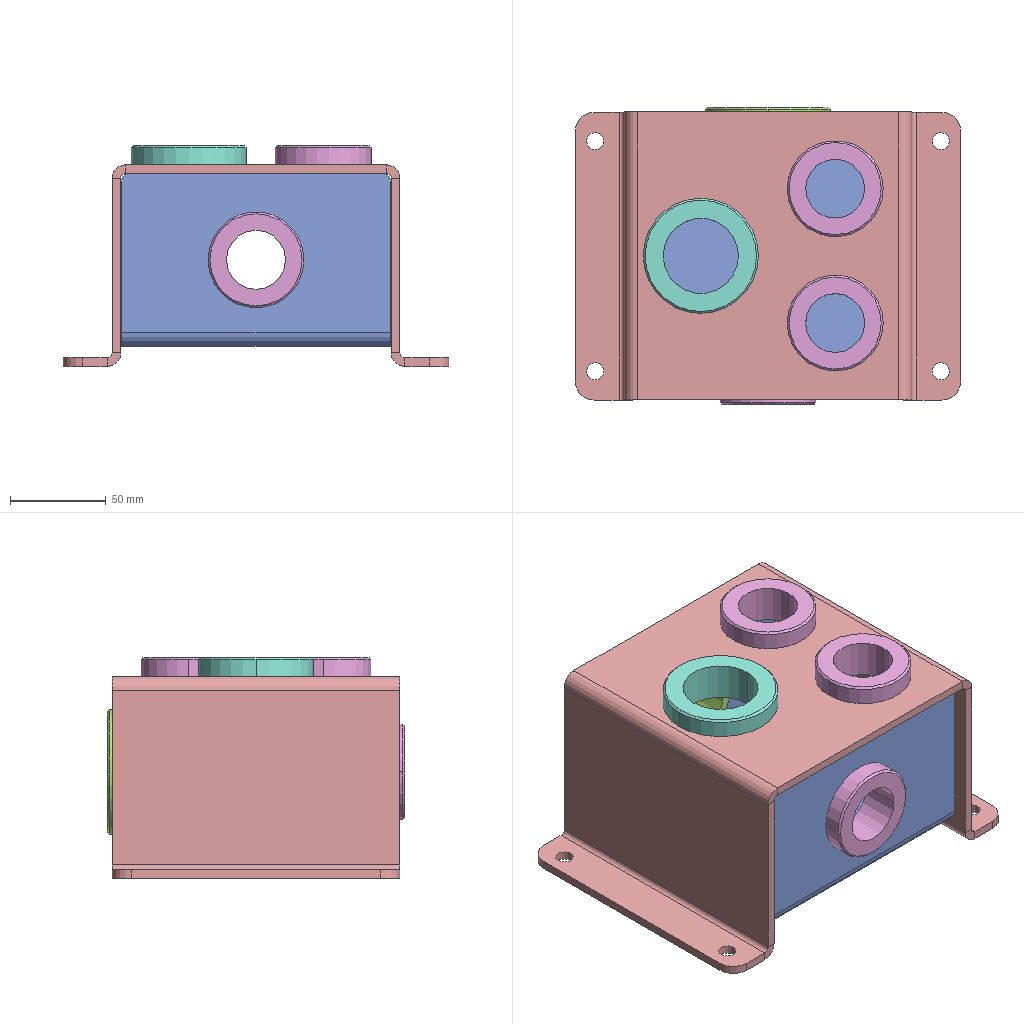Assembly | SolidWorks | 5 different items | 7 placed | box 201 x 155 x 115 mm
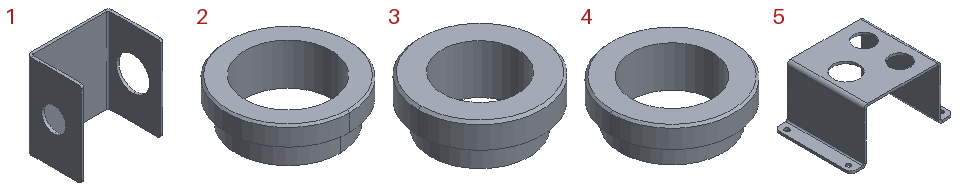Parts list (item | quantity | size | volume | features):
1 | x1 | 135 x 90 x 140 mm | 173803 mm3 | features Cut 2, Fillet 1, FlatPattern 1, SMBaseFlange 1, SheetMetal 1, UnFold 1
2 | x1 | 65 x 65 x 22 mm | 26213 mm3 | features Chamfer 1, HoleWzd 1, Revolution 1
3 | x3 | 50 x 50 x 20 mm | 17271 mm3 | features Chamfer 1, HoleWzd 1, Revolution 1
4 | x1 | 60 x 60 x 20 mm | 23617 mm3 | features Chamfer 1, HoleWzd 1, Revolution 1
5 | x1 | 201 x 150 x 105 mm | 244169 mm3 | features ICE 2, Fillet 1, FlatPattern 1, SMBaseFlange 1, SheetMetal 1, UnFold 1
Mates (type | each side: item.copy, entity, surface, feature):
Coincident | 1.1 face plane Base-Flange1 | 5.1 face plane Base-Flange1
DistanceDim | 1.1 face plane Base-Flange1 | 5.1 face plane Base-Flange1
Width | 1.1 face plane Base-Flange1 | 1.1 face plane Base-Flange1 | 5.1 face plane Base-Flange1 | 5.1 face plane Base-Flange1
Coincident | 1.1 face plane Base-Flange1 | 2.1 face plane Revolve1
Concentric | 1.1 face cylinder Cut-Extrude2 | 2.1 face cylinder Revolve1
Coincident | 5.1 face plane Base-Flange1 | 3.1 face plane Revolve1
Concentric | 3.1 face cylinder Revolve1 | 5.1 face cylinder Cut-Extrude2
Coincident | 5.1 face plane Base-Flange1 | 3.2 face plane Revolve1
Concentric | 3.2 face cylinder G1 Tapped Hole1 | 5.1 face cylinder Cut-Extrude2
Coincident | 5.1 face plane Base-Flange1 | 4.1 face plane Revolve1
Concentric | 4.1 face cylinder G1-1/4 Tapped Hole1 | 5.1 face cylinder Cut-Extrude2
Coincident | 1.1 face plane Base-Flange1 | 3.3 face plane Revolve1
Concentric | 1.1 face cylinder Cut-Extrude1 | 3.3 face cylinder G1 Tapped Hole1